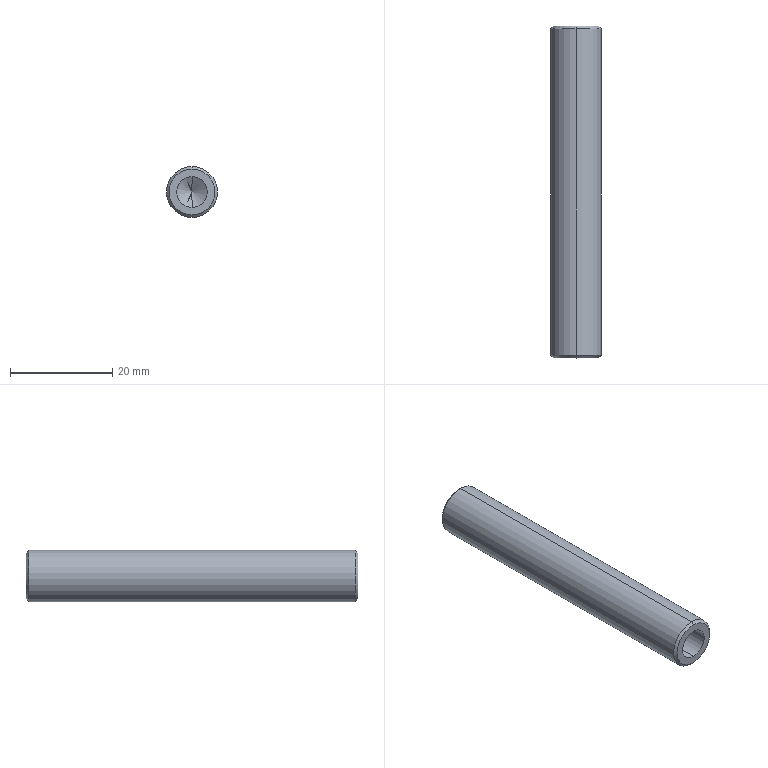Part | SolidWorks | features Chamfer 1, Extrusion 1, HoleWzd 1, MirrorPattern 1 | 1 solid | 16 faces | box 10 x 65 x 10 mm | volume 4498 mm3 | cone 8 | cylinder 6 | plane 2 | commonest cylinder face diameters 6 x4 10 x2
STEP:
#1=CARTESIAN_POINT('',(0.,0.,-4.5));
#2=VERTEX_POINT('',#1);
#3=CARTESIAN_POINT('',(0.,0.,4.5));
#4=VERTEX_POINT('',#3);
#5=CARTESIAN_POINT('',(0.,0.,0.));
#6=DIRECTION('',(0.,-1.,0.));
#7=DIRECTION('',(0.,0.,1.));
#8=AXIS2_PLACEMENT_3D('',#5,#6,#7);
#9=CIRCLE('',#8,4.5);
#10=EDGE_CURVE('',#2,#4,#9,.T.);
#11=ORIENTED_EDGE('',*,*,#10,.F.);
#12=CARTESIAN_POINT('',(0.,0.5,-5.));
#13=VERTEX_POINT('',#12);
#14=CARTESIAN_POINT('',(0.,0.5,-5.));
#15=DIRECTION('',(0.,0.7071,-0.7071));
#16=VECTOR('',#15,1000.);
#17=LINE('',#14,#16);
#18=EDGE_CURVE('',#2,#13,#17,.T.);
#19=ORIENTED_EDGE('',*,*,#18,.T.);
#20=CARTESIAN_POINT('',(0.,0.5,5.));
#21=VERTEX_POINT('',#20);
#22=CARTESIAN_POINT('',(0.,0.5,0.));
#23=DIRECTION('',(0.,1.,0.));
#24=DIRECTION('',(0.,0.,1.));
#25=AXIS2_PLACEMENT_3D('',#22,#23,#24);
#26=CIRCLE('',#25,5.);
#27=EDGE_CURVE('',#21,#13,#26,.T.);
#28=ORIENTED_EDGE('',*,*,#27,.F.);
#29=CARTESIAN_POINT('',(0.,0.5,5.));
#30=DIRECTION('',(0.,0.7071,0.7071));
#31=VECTOR('',#30,1000.);
#32=LINE('',#29,#31);
#33=EDGE_CURVE('',#4,#21,#32,.T.);
#34=ORIENTED_EDGE('',*,*,#33,.F.);
#35=EDGE_LOOP('',(#11,#19,#28,#34));
#36=FACE_OUTER_BOUND('',#35,.T.);
#37=CARTESIAN_POINT('',(0.,0.5,0.));
#38=DIRECTION('',(0.,1.,0.));
#39=DIRECTION('',(0.,0.,1.));
#40=AXIS2_PLACEMENT_3D('',#37,#38,#39);
#41=CONICAL_SURFACE('',#40,5.,0.7854);
#42=ADVANCED_FACE('',(#36),#41,.T.);
#43=CARTESIAN_POINT('',(0.,65.,4.5));
#44=VERTEX_POINT('',#43);
#45=CARTESIAN_POINT('',(0.,65.,-4.5));
#46=VERTEX_POINT('',#45);
#47=CARTESIAN_POINT('',(0.,65.,0.));
#48=DIRECTION('',(0.,1.,0.));
#49=DIRECTION('',(0.,0.,1.));
#50=AXIS2_PLACEMENT_3D('',#47,#48,#49);
#51=CIRCLE('',#50,4.5);
#52=EDGE_CURVE('',#44,#46,#51,.T.);
#53=ORIENTED_EDGE('',*,*,#52,.F.);
#54=CARTESIAN_POINT('',(0.,64.5,5.));
#55=VERTEX_POINT('',#54);
#56=CARTESIAN_POINT('',(0.,65.,4.5));
#57=DIRECTION('',(0.,-0.7071,0.7071));
#58=VECTOR('',#57,1000.);
#59=LINE('',#56,#58);
#60=EDGE_CURVE('',#44,#55,#59,.T.);
#61=ORIENTED_EDGE('',*,*,#60,.T.);
#62=CARTESIAN_POINT('',(0.,64.5,-5.));
#63=VERTEX_POINT('',#62);
#64=CARTESIAN_POINT('',(0.,64.5,0.));
#65=DIRECTION('',(0.,-1.,0.));
#66=DIRECTION('',(0.,0.,1.));
#67=AXIS2_PLACEMENT_3D('',#64,#65,#66);
#68=CIRCLE('',#67,5.);
#69=EDGE_CURVE('',#63,#55,#68,.T.);
#70=ORIENTED_EDGE('',*,*,#69,.F.);
#71=CARTESIAN_POINT('',(0.,65.,-4.5));
#72=DIRECTION('',(0.,-0.7071,-0.7071));
#73=VECTOR('',#72,1000.);
#74=LINE('',#71,#73);
#75=EDGE_CURVE('',#46,#63,#74,.T.);
#76=ORIENTED_EDGE('',*,*,#75,.F.);
#77=EDGE_LOOP('',(#53,#61,#70,#76));
#78=FACE_OUTER_BOUND('',#77,.T.);
#79=CARTESIAN_POINT('',(0.,65.,0.));
#80=DIRECTION('',(0.,-1.,0.));
#81=DIRECTION('',(0.,0.,-1.));
#82=AXIS2_PLACEMENT_3D('',#79,#80,#81);
#83=CONICAL_SURFACE('',#82,4.5,0.7854);
#84=ADVANCED_FACE('',(#78),#83,.T.);
#85=CARTESIAN_POINT('',(0.,10.,3.));
#86=VERTEX_POINT('',#85);
#87=CARTESIAN_POINT('',(0.,10.,-3.));
#88=VERTEX_POINT('',#87);
#89=CARTESIAN_POINT('',(0.,10.,0.));
#90=DIRECTION('',(0.,-1.,0.));
#91=DIRECTION('',(0.,0.,-1.));
#92=AXIS2_PLACEMENT_3D('',#89,#90,#91);
#93=CIRCLE('',#92,3.);
#94=EDGE_CURVE('',#86,#88,#93,.T.);
#95=ORIENTED_EDGE('',*,*,#94,.F.);
#96=CARTESIAN_POINT('',(0.,0.,3.));
#97=VERTEX_POINT('',#96);
#98=CARTESIAN_POINT('',(0.,0.,3.));
#99=DIRECTION('',(0.,-1.,0.));
#100=VECTOR('',#99,1000.);
#101=LINE('',#98,#100);
#102=EDGE_CURVE('',#86,#97,#101,.T.);
#103=ORIENTED_EDGE('',*,*,#102,.T.);
#104=CARTESIAN_POINT('',(0.,0.,-3.));
#105=VERTEX_POINT('',#104);
#106=CARTESIAN_POINT('',(0.,0.,0.));
#107=DIRECTION('',(0.,-1.,0.));
#108=DIRECTION('',(0.,0.,-1.));
#109=AXIS2_PLACEMENT_3D('',#106,#107,#108);
#110=CIRCLE('',#109,3.);
#111=EDGE_CURVE('',#97,#105,#110,.T.);
#112=ORIENTED_EDGE('',*,*,#111,.T.);
#113=CARTESIAN_POINT('',(0.,0.,-3.));
#114=DIRECTION('',(0.,-1.,0.));
#115=VECTOR('',#114,1000.);
#116=LINE('',#113,#115);
#117=EDGE_CURVE('',#88,#105,#116,.T.);
#118=ORIENTED_EDGE('',*,*,#117,.F.);
#119=EDGE_LOOP('',(#95,#103,#112,#118));
#120=FACE_OUTER_BOUND('',#119,.T.);
#121=CARTESIAN_POINT('',(0.,0.,0.));
#122=DIRECTION('',(0.,-1.,0.));
#123=DIRECTION('',(0.,0.,-1.));
#124=AXIS2_PLACEMENT_3D('',#121,#122,#123);
#125=CYLINDRICAL_SURFACE('',#124,3.);
#126=ADVANCED_FACE('',(#120),#125,.F.);
#127=CARTESIAN_POINT('',(0.,11.803,0.));
#128=VERTEX_POINT('',#127);
#129=CARTESIAN_POINT('',(0.,10.,-3.));
#130=DIRECTION('',(0.,-0.515,-0.8572));
#131=VECTOR('',#130,1000.);
#132=LINE('',#129,#131);
#133=EDGE_CURVE('',#128,#88,#132,.T.);
#134=ORIENTED_EDGE('',*,*,#133,.F.);
#135=CARTESIAN_POINT('',(0.,10.,3.));
#136=DIRECTION('',(0.,-0.515,0.8572));
#137=VECTOR('',#136,1000.);
#138=LINE('',#135,#137);
#139=EDGE_CURVE('',#128,#86,#138,.T.);
#140=ORIENTED_EDGE('',*,*,#139,.T.);
#141=ORIENTED_EDGE('',*,*,#94,.T.);
#142=EDGE_LOOP('',(#134,#140,#141));
#143=FACE_OUTER_BOUND('',#142,.T.);
#144=CARTESIAN_POINT('',(0.,10.,0.));
#145=DIRECTION('',(0.,-1.,0.));
#146=DIRECTION('',(0.,0.,-1.));
#147=AXIS2_PLACEMENT_3D('',#144,#145,#146);
#148=CONICAL_SURFACE('',#147,3.,1.03);
#149=ADVANCED_FACE('',(#143),#148,.F.);
#150=CARTESIAN_POINT('',(0.,55.,-3.));
#151=VERTEX_POINT('',#150);
#152=CARTESIAN_POINT('',(0.,55.,3.));
#153=VERTEX_POINT('',#152);
#154=CARTESIAN_POINT('',(0.,55.,0.));
#155=DIRECTION('',(0.,1.,0.));
#156=DIRECTION('',(0.,0.,1.));
#157=AXIS2_PLACEMENT_3D('',#154,#155,#156);
#158=CIRCLE('',#157,3.);
#159=EDGE_CURVE('',#151,#153,#158,.T.);
#160=ORIENTED_EDGE('',*,*,#159,.F.);
#161=CARTESIAN_POINT('',(0.,65.,-3.));
#162=VERTEX_POINT('',#161);
#163=CARTESIAN_POINT('',(0.,65.,-3.));
#164=DIRECTION('',(0.,1.,0.));
#165=VECTOR('',#164,1000.);
#166=LINE('',#163,#165);
#167=EDGE_CURVE('',#151,#162,#166,.T.);
#168=ORIENTED_EDGE('',*,*,#167,.T.);
#169=CARTESIAN_POINT('',(0.,65.,3.));
#170=VERTEX_POINT('',#169);
#171=CARTESIAN_POINT('',(0.,65.,0.));
#172=DIRECTION('',(0.,1.,0.));
#173=DIRECTION('',(0.,0.,1.));
#174=AXIS2_PLACEMENT_3D('',#171,#172,#173);
#175=CIRCLE('',#174,3.);
#176=EDGE_CURVE('',#162,#170,#175,.T.);
#177=ORIENTED_EDGE('',*,*,#176,.T.);
#178=CARTESIAN_POINT('',(0.,65.,3.));
#179=DIRECTION('',(0.,1.,0.));
#180=VECTOR('',#179,1000.);
#181=LINE('',#178,#180);
#182=EDGE_CURVE('',#153,#170,#181,.T.);
#183=ORIENTED_EDGE('',*,*,#182,.F.);
#184=EDGE_LOOP('',(#160,#168,#177,#183));
#185=FACE_OUTER_BOUND('',#184,.T.);
#186=CARTESIAN_POINT('',(0.,65.,0.));
#187=DIRECTION('',(0.,1.,0.));
#188=DIRECTION('',(0.,0.,1.));
#189=AXIS2_PLACEMENT_3D('',#186,#187,#188);
#190=CYLINDRICAL_SURFACE('',#189,3.);
#191=ADVANCED_FACE('',(#185),#190,.F.);
#192=CARTESIAN_POINT('',(0.,53.197,0.));
#193=VERTEX_POINT('',#192);
#194=CARTESIAN_POINT('',(0.,55.,3.));
#195=DIRECTION('',(0.,0.515,0.8572));
#196=VECTOR('',#195,1000.);
#197=LINE('',#194,#196);
#198=EDGE_CURVE('',#193,#153,#197,.T.);
#199=ORIENTED_EDGE('',*,*,#198,.F.);
#200=CARTESIAN_POINT('',(0.,55.,-3.));
#201=DIRECTION('',(0.,0.515,-0.8572));
#202=VECTOR('',#201,1000.);
#203=LINE('',#200,#202);
#204=EDGE_CURVE('',#193,#151,#203,.T.);
#205=ORIENTED_EDGE('',*,*,#204,.T.);
#206=ORIENTED_EDGE('',*,*,#159,.T.);
#207=EDGE_LOOP('',(#199,#205,#206));
#208=FACE_OUTER_BOUND('',#207,.T.);
#209=CARTESIAN_POINT('',(0.,55.,0.));
#210=DIRECTION('',(0.,1.,0.));
#211=DIRECTION('',(0.,0.,1.));
#212=AXIS2_PLACEMENT_3D('',#209,#210,#211);
#213=CONICAL_SURFACE('',#212,3.,1.03);
#214=ADVANCED_FACE('',(#208),#213,.F.);
#215=ORIENTED_EDGE('',*,*,#69,.T.);
#216=CARTESIAN_POINT('',(0.,65.,5.));
#217=DIRECTION('',(0.,-1.,0.));
#218=VECTOR('',#217,1000.);
#219=LINE('',#216,#218);
#220=EDGE_CURVE('',#55,#21,#219,.T.);
#221=ORIENTED_EDGE('',*,*,#220,.T.);
#222=ORIENTED_EDGE('',*,*,#27,.T.);
#223=CARTESIAN_POINT('',(0.,65.,-5.));
#224=DIRECTION('',(0.,-1.,0.));
#225=VECTOR('',#224,1000.);
#226=LINE('',#223,#225);
#227=EDGE_CURVE('',#63,#13,#226,.T.);
#228=ORIENTED_EDGE('',*,*,#227,.F.);
#229=EDGE_LOOP('',(#215,#221,#222,#228));
#230=FACE_OUTER_BOUND('',#229,.T.);
#231=CARTESIAN_POINT('',(0.,65.,0.));
#232=DIRECTION('',(0.,-1.,0.));
#233=DIRECTION('',(0.,0.,-1.));
#234=AXIS2_PLACEMENT_3D('',#231,#232,#233);
#235=CYLINDRICAL_SURFACE('',#234,5.);
#236=ADVANCED_FACE('',(#230),#235,.T.);
#237=ORIENTED_EDGE('',*,*,#220,.F.);
#238=CARTESIAN_POINT('',(0.,64.5,0.));
#239=DIRECTION('',(0.,-1.,0.));
#240=DIRECTION('',(0.,0.,1.));
#241=AXIS2_PLACEMENT_3D('',#238,#239,#240);
#242=CIRCLE('',#241,5.);
#243=EDGE_CURVE('',#55,#63,#242,.T.);
#244=ORIENTED_EDGE('',*,*,#243,.T.);
#245=ORIENTED_EDGE('',*,*,#227,.T.);
#246=CARTESIAN_POINT('',(0.,0.5,0.));
#247=DIRECTION('',(0.,1.,0.));
#248=DIRECTION('',(0.,0.,1.));
#249=AXIS2_PLACEMENT_3D('',#246,#247,#248);
#250=CIRCLE('',#249,5.);
#251=EDGE_CURVE('',#13,#21,#250,.T.);
#252=ORIENTED_EDGE('',*,*,#251,.T.);
#253=EDGE_LOOP('',(#237,#244,#245,#252));
#254=FACE_OUTER_BOUND('',#253,.T.);
#255=CARTESIAN_POINT('',(0.,65.,0.));
#256=DIRECTION('',(0.,-1.,0.));
#257=DIRECTION('',(0.,0.,-1.));
#258=AXIS2_PLACEMENT_3D('',#255,#256,#257);
#259=CYLINDRICAL_SURFACE('',#258,5.);
#260=ADVANCED_FACE('',(#254),#259,.T.);
#261=CARTESIAN_POINT('',(0.,65.,0.));
#262=DIRECTION('',(0.,1.,0.));
#263=DIRECTION('',(0.,0.,1.));
#264=AXIS2_PLACEMENT_3D('',#261,#262,#263);
#265=CIRCLE('',#264,4.5);
#266=EDGE_CURVE('',#46,#44,#265,.T.);
#267=ORIENTED_EDGE('',*,*,#266,.T.);
#268=ORIENTED_EDGE('',*,*,#52,.T.);
#269=EDGE_LOOP('',(#267,#268));
#270=FACE_OUTER_BOUND('',#269,.T.);
#271=CARTESIAN_POINT('',(0.,65.,0.));
#272=DIRECTION('',(0.,1.,0.));
#273=DIRECTION('',(0.,0.,1.));
#274=AXIS2_PLACEMENT_3D('',#271,#272,#273);
#275=CIRCLE('',#274,3.);
#276=EDGE_CURVE('',#170,#162,#275,.T.);
#277=ORIENTED_EDGE('',*,*,#276,.F.);
#278=ORIENTED_EDGE('',*,*,#176,.F.);
#279=EDGE_LOOP('',(#277,#278));
#280=FACE_BOUND('',#279,.T.);
#281=CARTESIAN_POINT('',(0.,65.,0.));
#282=DIRECTION('',(0.,1.,0.));
#283=DIRECTION('',(0.,0.,1.));
#284=AXIS2_PLACEMENT_3D('',#281,#282,#283);
#285=PLANE('',#284);
#286=ADVANCED_FACE('',(#270,#280),#285,.T.);
#287=CARTESIAN_POINT('',(0.,0.,0.));
#288=DIRECTION('',(0.,-1.,0.));
#289=DIRECTION('',(0.,0.,1.));
#290=AXIS2_PLACEMENT_3D('',#287,#288,#289);
#291=CIRCLE('',#290,4.5);
#292=EDGE_CURVE('',#4,#2,#291,.T.);
#293=ORIENTED_EDGE('',*,*,#292,.T.);
#294=ORIENTED_EDGE('',*,*,#10,.T.);
#295=EDGE_LOOP('',(#293,#294));
#296=FACE_OUTER_BOUND('',#295,.T.);
#297=CARTESIAN_POINT('',(0.,0.,0.));
#298=DIRECTION('',(0.,-1.,0.));
#299=DIRECTION('',(0.,0.,-1.));
#300=AXIS2_PLACEMENT_3D('',#297,#298,#299);
#301=CIRCLE('',#300,3.);
#302=EDGE_CURVE('',#105,#97,#301,.T.);
#303=ORIENTED_EDGE('',*,*,#302,.F.);
#304=ORIENTED_EDGE('',*,*,#111,.F.);
#305=EDGE_LOOP('',(#303,#304));
#306=FACE_BOUND('',#305,.T.);
#307=CARTESIAN_POINT('',(0.,0.,0.));
#308=DIRECTION('',(0.,1.,0.));
#309=DIRECTION('',(0.,0.,1.));
#310=AXIS2_PLACEMENT_3D('',#307,#308,#309);
#311=PLANE('',#310);
#312=ADVANCED_FACE('',(#296,#306),#311,.F.);
#313=ORIENTED_EDGE('',*,*,#204,.F.);
#314=ORIENTED_EDGE('',*,*,#198,.T.);
#315=CARTESIAN_POINT('',(0.,55.,0.));
#316=DIRECTION('',(0.,1.,0.));
#317=DIRECTION('',(0.,0.,1.));
#318=AXIS2_PLACEMENT_3D('',#315,#316,#317);
#319=CIRCLE('',#318,3.);
#320=EDGE_CURVE('',#153,#151,#319,.T.);
#321=ORIENTED_EDGE('',*,*,#320,.T.);
#322=EDGE_LOOP('',(#313,#314,#321));
#323=FACE_OUTER_BOUND('',#322,.T.);
#324=CARTESIAN_POINT('',(0.,55.,0.));
#325=DIRECTION('',(0.,1.,0.));
#326=DIRECTION('',(0.,0.,1.));
#327=AXIS2_PLACEMENT_3D('',#324,#325,#326);
#328=CONICAL_SURFACE('',#327,3.,1.03);
#329=ADVANCED_FACE('',(#323),#328,.F.);
#330=ORIENTED_EDGE('',*,*,#167,.F.);
#331=ORIENTED_EDGE('',*,*,#320,.F.);
#332=ORIENTED_EDGE('',*,*,#182,.T.);
#333=ORIENTED_EDGE('',*,*,#276,.T.);
#334=EDGE_LOOP('',(#330,#331,#332,#333));
#335=FACE_OUTER_BOUND('',#334,.T.);
#336=CARTESIAN_POINT('',(0.,65.,0.));
#337=DIRECTION('',(0.,1.,0.));
#338=DIRECTION('',(0.,0.,1.));
#339=AXIS2_PLACEMENT_3D('',#336,#337,#338);
#340=CYLINDRICAL_SURFACE('',#339,3.);
#341=ADVANCED_FACE('',(#335),#340,.F.);
#342=ORIENTED_EDGE('',*,*,#139,.F.);
#343=ORIENTED_EDGE('',*,*,#133,.T.);
#344=CARTESIAN_POINT('',(0.,10.,0.));
#345=DIRECTION('',(0.,-1.,0.));
#346=DIRECTION('',(0.,0.,-1.));
#347=AXIS2_PLACEMENT_3D('',#344,#345,#346);
#348=CIRCLE('',#347,3.);
#349=EDGE_CURVE('',#88,#86,#348,.T.);
#350=ORIENTED_EDGE('',*,*,#349,.T.);
#351=EDGE_LOOP('',(#342,#343,#350));
#352=FACE_OUTER_BOUND('',#351,.T.);
#353=CARTESIAN_POINT('',(0.,10.,0.));
#354=DIRECTION('',(0.,-1.,0.));
#355=DIRECTION('',(0.,0.,-1.));
#356=AXIS2_PLACEMENT_3D('',#353,#354,#355);
#357=CONICAL_SURFACE('',#356,3.,1.03);
#358=ADVANCED_FACE('',(#352),#357,.F.);
#359=ORIENTED_EDGE('',*,*,#102,.F.);
#360=ORIENTED_EDGE('',*,*,#349,.F.);
#361=ORIENTED_EDGE('',*,*,#117,.T.);
#362=ORIENTED_EDGE('',*,*,#302,.T.);
#363=EDGE_LOOP('',(#359,#360,#361,#362));
#364=FACE_OUTER_BOUND('',#363,.T.);
#365=CARTESIAN_POINT('',(0.,0.,0.));
#366=DIRECTION('',(0.,-1.,0.));
#367=DIRECTION('',(0.,0.,-1.));
#368=AXIS2_PLACEMENT_3D('',#365,#366,#367);
#369=CYLINDRICAL_SURFACE('',#368,3.);
#370=ADVANCED_FACE('',(#364),#369,.F.);
#371=ORIENTED_EDGE('',*,*,#60,.F.);
#372=ORIENTED_EDGE('',*,*,#266,.F.);
#373=ORIENTED_EDGE('',*,*,#75,.T.);
#374=ORIENTED_EDGE('',*,*,#243,.F.);
#375=EDGE_LOOP('',(#371,#372,#373,#374));
#376=FACE_OUTER_BOUND('',#375,.T.);
#377=CARTESIAN_POINT('',(0.,65.,0.));
#378=DIRECTION('',(0.,-1.,0.));
#379=DIRECTION('',(0.,0.,-1.));
#380=AXIS2_PLACEMENT_3D('',#377,#378,#379);
#381=CONICAL_SURFACE('',#380,4.5,0.7854);
#382=ADVANCED_FACE('',(#376),#381,.T.);
#383=ORIENTED_EDGE('',*,*,#18,.F.);
#384=ORIENTED_EDGE('',*,*,#292,.F.);
#385=ORIENTED_EDGE('',*,*,#33,.T.);
#386=ORIENTED_EDGE('',*,*,#251,.F.);
#387=EDGE_LOOP('',(#383,#384,#385,#386));
#388=FACE_OUTER_BOUND('',#387,.T.);
#389=CARTESIAN_POINT('',(0.,0.5,0.));
#390=DIRECTION('',(0.,1.,0.));
#391=DIRECTION('',(0.,0.,1.));
#392=AXIS2_PLACEMENT_3D('',#389,#390,#391);
#393=CONICAL_SURFACE('',#392,5.,0.7854);
#394=ADVANCED_FACE('',(#388),#393,.T.);
#395=CLOSED_SHELL('',(#42,#84,#126,#149,#191,#214,#236,#260,#286,#312,#329,#341,#358,#370,#382,#394));
#396=MANIFOLD_SOLID_BREP('',#395);
#397=CARTESIAN_POINT('',(0.,0.,0.));
#398=DIRECTION('',(0.,0.,1.));
#399=DIRECTION('',(1.,0.,0.));
#400=AXIS2_PLACEMENT_3D('',#397,#398,#399);
#401=(LENGTH_UNIT()NAMED_UNIT(*)SI_UNIT(.MILLI.,.METRE.));
#402=UNCERTAINTY_MEASURE_WITH_UNIT(LENGTH_MEASURE(0.00001),#401,'','');
#403=(NAMED_UNIT(*)PLANE_ANGLE_UNIT()SI_UNIT($,.RADIAN.));
#404=(NAMED_UNIT(*)SI_UNIT($,.STERADIAN.)SOLID_ANGLE_UNIT());
#405=(GEOMETRIC_REPRESENTATION_CONTEXT(3)GLOBAL_UNCERTAINTY_ASSIGNED_CONTEXT((#402))GLOBAL_UNIT_ASSIGNED_CONTEXT((#401,#403,#404))REPRESENTATION_CONTEXT('',''));
#406=ADVANCED_BREP_SHAPE_REPRESENTATION('',(#396,#400),#405);